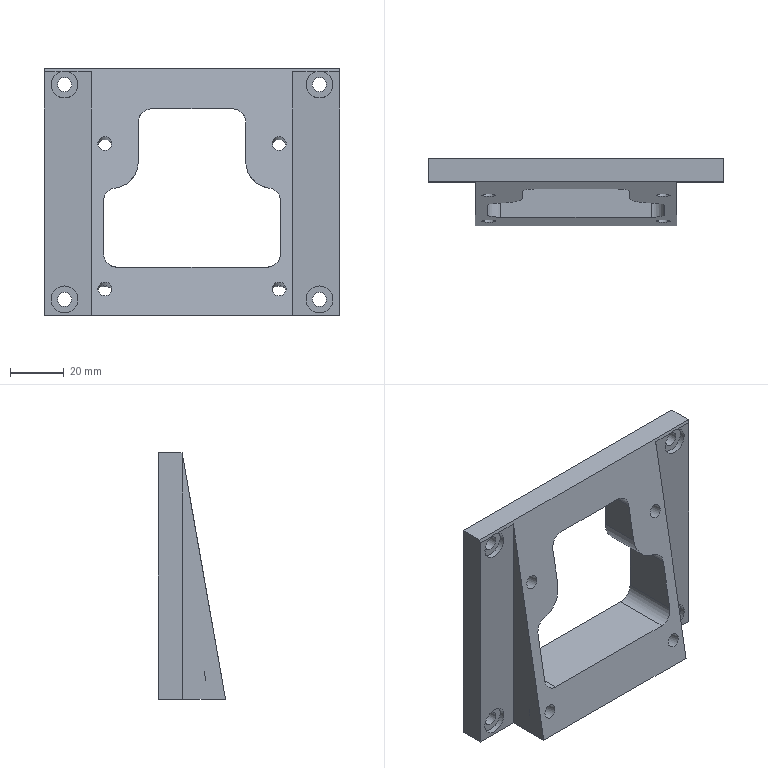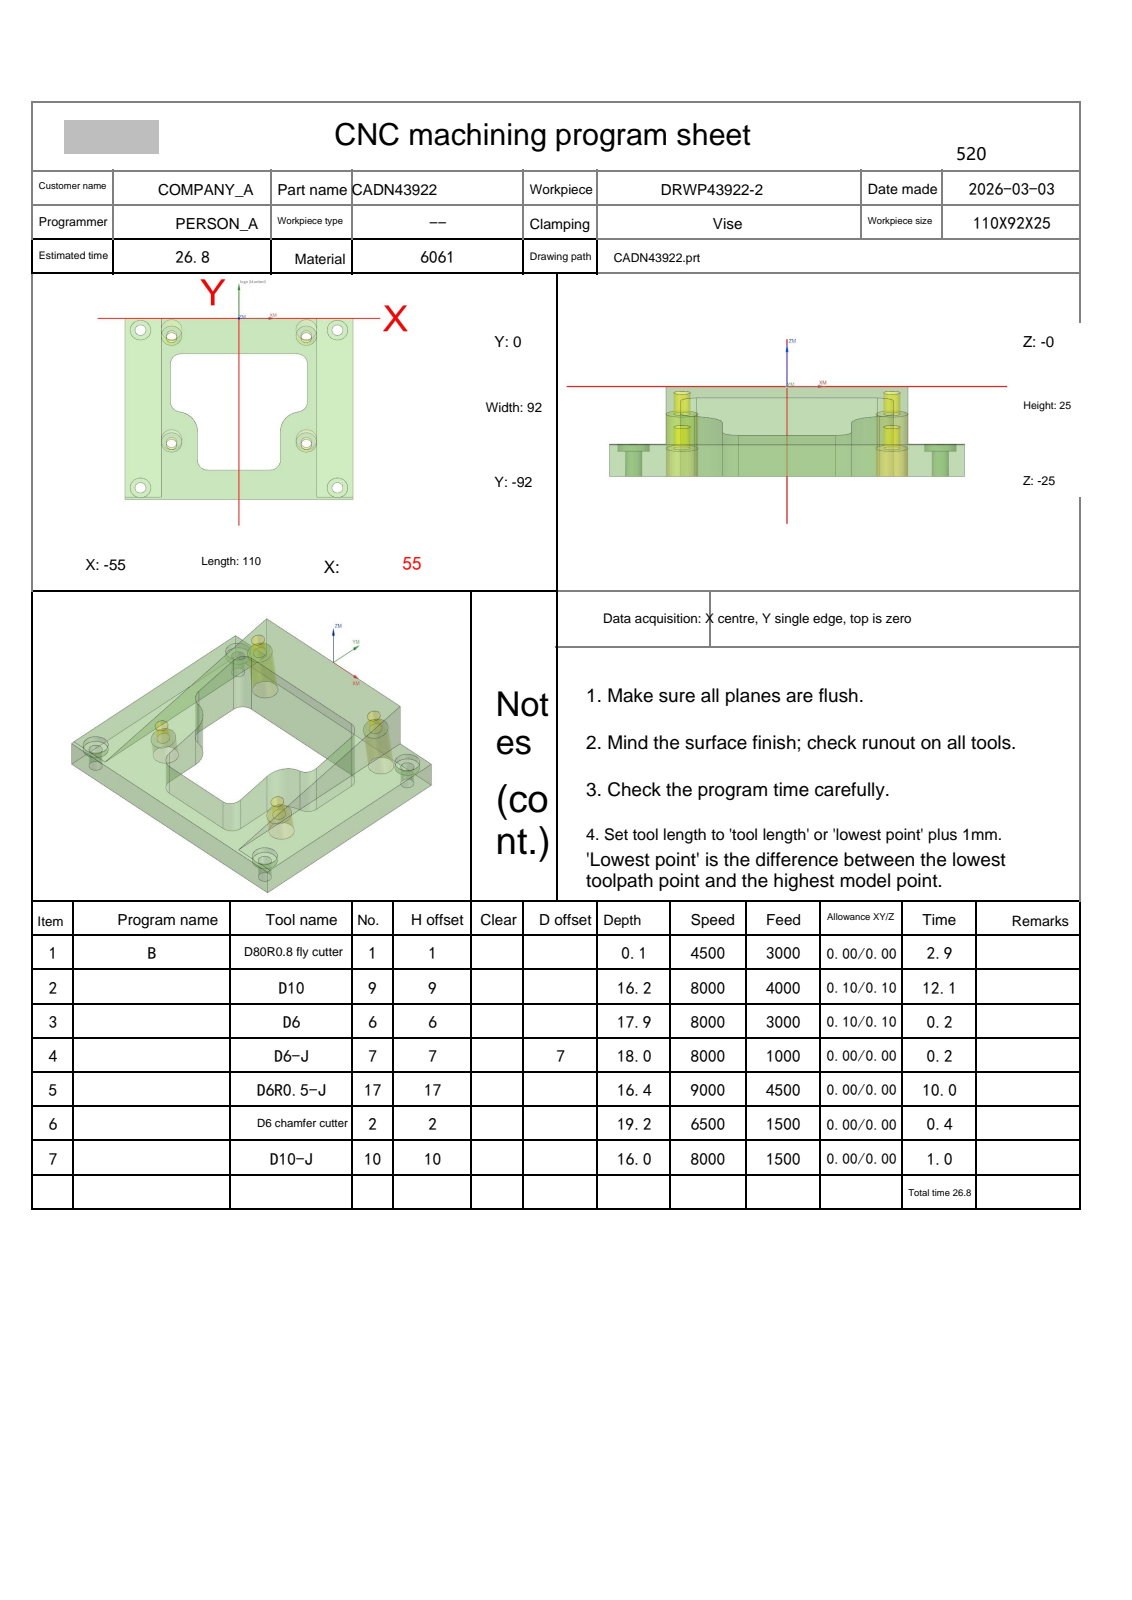NC program | NX | posted by the shop | part box 110 x 25 x 92 mm
Lines 183 to 1230 of 14355:
N2 T09 M06
(D10  D=10. R=0. H=09 ce=0.10 di=0.10)
G00 G90 G54 X7. Y-108. M03 S8000
G43 H09 Z14.5
M08
Z.509
G01 Z-.691 F4000.
Y-103.5
G03 X0.0 Y-96.5 I-7. J0.0
G01 X-51.
X-57.495
X-57.5
G02 X-58.003 Y-95.997 I0.0 J.503
G01 X-58. Y-95.943
X-58.001 Y3.993
Y3.998
G02 X-57.497 Y4.502 I.504 J0.0
G01 X-57.454 Y4.5
X-42.19
G02 X-37.512 Y6.5 I4.69 J-4.5
G01 X37.638 Y6.499
G02 X42.19 Y4.5 I-.138 J-6.499
G01 X57.495
X57.499
G02 X58.004 Y3.996 I0.0 J-.504
G01 X58.001 Y3.943
Y-95.994
Y-95.999
G02 X57.498 Y-96.502 I-.503 J0.0
G01 X57.454 Y-96.5
X-1.986
G02 X-2.799 Y-96.082 I.001 J1.
G01 X-7.201 Y-89.918
G03 X-8.014 Y-89.5 I-.813 J-.582
G01 X-50.003
G02 X-51. Y-88.502 I.002 J1.
G01 X-51.001 Y-11.861
G02 X-50.735 Y-11.182 I1. J0.0
G01 X-49.575 Y-9.925
G03 X-49.317 Y-9.373 I-.735 J.678
G02 X-46.837 Y-7.188 I2.48 J-.315
X-44.494 Y-8.817 I0.0 J-2.5
G01 X-42.645 Y-13.789
G02 X-42.488 Y-14.661 I-2.343 J-.871
X-44.988 Y-17.161 I-2.5 J0.0
X-47.331 Y-15.532 I0.0 J2.5
G01 X-48.77 Y-11.664
G03 X-49.071 Y-11.241 I-.937 J-.349
G01 X-50.637 Y-9.949
G02 X-51.001 Y-9.178 I.636 J.771
G01 Y-3.498
G02 X-50.003 Y-2.5 I1. J-.002
G01 X-44.998
G02 X-44. Y-3.497 I-.002 J-1.
G01 Y-3.904
X-44.002 Y-4.056
G03 X-37.5 Y-10.896 I6.849 J0.0
G01 X37.597 Y-10.893
G03 X44.001 Y-4.029 I-.476 J6.864
G01 Y-3.986
G03 X43.556 Y-3.287 I-.779 J-.005
G01 X43.2 Y-3.118
X43.02 Y-3.078
G03 X42.6 Y-3.498 I0.0 J-.42
G01 Y-3.921
X42.601 Y-4.029
G02 X37.5 Y-9.496 I-5.48 J0.0
G01 X-37.5
G02 X-42.602 Y-4.059 I.347 J5.438
G01 X-42.6 Y-3.921
Y-.444
G02 X-42.608 Y-.14 I5.438 J.304
X-42.592 Y.278 I5.446 J0.0
X-37.512 Y5.1 I5.093 J-.278
G01 X37.608 Y5.099
G02 X42.063 Y2.279 I-.108 J-5.099
X42.611 Y-.028 I-4.58 J-2.306
X42.6 Y-.356 I-5.128 J0.0
G01 Y-3.498
G03 X43.02 Y-3.918 I.42 J0.0
G01 X43.2 Y-3.877
X43.797 Y-3.594
G03 X44.018 Y-3.309 I-.172 J.361
G02 X44.998 Y-2.5 I.982 J-.191
G01 X50.003
G02 X51.001 Y-3.498 I-.002 J-1.
G01 Y-9.161
G02 X50.637 Y-9.932 I-1. J0.0
G01 X49.07 Y-11.225
G03 X48.769 Y-11.648 I.637 J-.771
G01 X47.329 Y-15.524
G02 X44.986 Y-17.153 I-2.343 J.871
X42.486 Y-14.653 I0.0 J2.5
X42.643 Y-13.782 I2.5 J0.0
G01 X44.493 Y-8.801
G02 X46.837 Y-7.172 I2.343 J-.871
X49.316 Y-9.356 I0.0 J-2.5
G03 X49.574 Y-9.908 I.992 J.126
G01 X50.735 Y-11.165
G02 X51.001 Y-11.844 I-.735 J-.678
G01 X51. Y-88.503
G02 X50.003 Y-89.5 I-1. J.002
G01 X-1.986
G02 X-2.799 Y-89.082 I.001 J1.
G01 X-7.201 Y-82.918
G03 X-8.014 Y-82.5 I-.813 J-.582
G01 X-43.003
G02 X-44. Y-81.503 I.003 J1.
G01 X-44.001 Y-17.703
G02 X-43.001 Y-16.705 I1. J-.003
X-42.609 Y-16.785 I0.0 J-1.
G03 X-37.678 Y-17.896 I5.459 J12.727
G01 X37.5
G03 X38.081 Y-17.876 I0.0 J8.4
X42.608 Y-16.779 I-.96 J13.847
G02 X43.001 Y-16.699 I.393 J-.92
X44.001 Y-17.696 I0.0 J-1.
G01 X44. Y-81.503
G02 X43.003 Y-82.5 I-1. J.003
G01 X-1.986
G02 X-2.799 Y-82.082 I.001 J1.
G01 X-7.201 Y-75.919
G03 X-8.014 Y-75.5 I-.813 J-.582
G01 X-36.003
G02 X-37. Y-74.503 I.003 J1.
G01 X-37.001 Y-25.893
G02 X-36.004 Y-24.896 I1. J-.003
G01 X36.004
G02 X37.001 Y-25.893 I-.003 J-1.
G01 X37. Y-74.503
G02 X36.003 Y-75.5 I-1. J.003
G01 X-1.986
G02 X-2.799 Y-75.082 I.001 J1.
G01 X-7.201 Y-68.919
G03 X-8.014 Y-68.5 I-.813 J-.582
G01 X-29.004
G02 X-30. Y-67.503 I.003 J1.
G01 X-30.001 Y-32.893
G02 X-29.004 Y-31.896 I1. J-.003
G01 X29.004
G02 X30.001 Y-32.893 I-.003 J-1.
G01 X30. Y-67.504
G02 X29.004 Y-68.5 I-1. J.003
G01 X-1.986
G02 X-2.799 Y-68.082 I0.0 J1.
G01 X-7.201 Y-61.919
G03 X-8.014 Y-61.5 I-.814 J-.582
G01 X-22.004
G02 X-23. Y-60.504 I.004 J1.
G01 X-23.001 Y-39.893
G02 X-22.004 Y-38.896 I1. J-.004
G01 X22.004
G02 X23.001 Y-39.893 I-.004 J-1.
G01 X23. Y-60.504
G02 X22.004 Y-61.5 I-1. J.004
G01 X-1.986
G02 X-2.799 Y-61.082 I0.0 J1.
G01 X-7.201 Y-54.919
G03 X-8.014 Y-54.5 I-.814 J-.582
G01 X-15.004
G02 X-16.001 Y-53.504 I.004 J1.
G01 Y-46.893
G02 X-15.004 Y-45.896 I1. J-.004
G01 X15.004
G02 X16.001 Y-46.893 I-.004 J-1.
G01 Y-53.504
G02 X15.004 Y-54.5 I-1. J.004
G01 X-5.
X-5.5
G03 X-12.5 Y-61.5 I0.0 J-7.
G01 Z.509
G00 Z3.
G01 X7. Y-108. F6000.
G00 Z-.183
G01 Z-1.383 F4000.
Y-103.5
G03 X0.0 Y-96.5 I-7. J0.0
G01 X-51.
X-57.495
X-57.5
G02 X-58.003 Y-95.997 I0.0 J.503
G01 X-58. Y-95.943
X-58.001 Y3.993
Y3.998
G02 X-57.497 Y4.502 I.504 J0.0
G01 X-57.454 Y4.5
X-42.19
G02 X-37.512 Y6.5 I4.69 J-4.5
G01 X37.628 Y6.499
G02 X42.19 Y4.5 I-.128 J-6.499
G01 X57.495
X57.499
G02 X58.004 Y3.996 I0.0 J-.504
G01 X58.001 Y3.943
Y-95.994
Y-95.999
G02 X57.498 Y-96.502 I-.503 J0.0
G01 X57.454 Y-96.5
X-5.
G02 X-5.971 Y-95.738 I0.0 J1.
G01 X-7.313 Y-90.262
G03 X-8.284 Y-89.5 I-.971 J-.239
G01 X-50.003
G02 X-51. Y-88.503 I.002 J1.
G01 X-51.001 Y-15.949
G02 X-50.736 Y-15.271 I1. J0.0
G01 X-49.576 Y-14.015
G03 X-49.319 Y-13.463 I-.735 J.678
G02 X-46.839 Y-11.276 I2.48 J-.313
X-44.496 Y-12.903 I0.0 J-2.5
G01 X-42.664 Y-17.819
G02 X-42.507 Y-18.692 I-2.343 J-.873
X-45.007 Y-21.192 I-2.5 J0.0
X-47.349 Y-19.565 I0.0 J2.5
G01 X-48.77 Y-15.753
G03 X-49.071 Y-15.33 I-.937 J-.349
G01 X-50.637 Y-14.039
G02 X-51.001 Y-13.268 I.636 J.772
G01 Y-3.497
G02 X-50.003 Y-2.5 I1. J-.002
G01 X-44.998
G02 X-44. Y-3.497 I-.002 J-1.
G01 Y-3.904
X-44.002 Y-4.059
X-44. Y-4.213
X-43.999 Y-7.906
X-43.973 Y-8.386
X-43.867 Y-9.275
G03 X-37.501 Y-14.817 I6.371 J.892
G01 X-34.608
G03 X-32.75 Y-14.55 I-.076 J7.123
G02 X-32.481 Y-14.513 I.269 J-.963
X-32.179 Y-14.56 I0.0 J-1.
G01 X-32.04 Y-14.604
G03 X-31.818 Y-14.656 I.427 J1.333
G01 X-30.927 Y-14.787
X-30.787 Y-14.8
X-30.392 Y-14.817
X30.456 Y-14.816
X30.787 Y-14.8
X30.93 Y-14.786
X31.82 Y-14.654
G03 X32.036 Y-14.604 I-.207 J1.385
G01 X32.177 Y-14.559
G02 X32.476 Y-14.513 I.299 J-.954
X32.746 Y-14.55 I0.0 J-1.
G03 X34.608 Y-14.817 I1.928 J6.82
G01 X37.5
G03 X44.004 Y-7.954 I-.37 J6.863
X44. Y-7.731 I-6.873 J0.0
G01 Y-4.151
X44.001 Y-3.985
G03 X43.556 Y-3.287 I-.779 J-.005
G01 X43.2 Y-3.118
X43.02 Y-3.077
G03 X42.6 Y-3.497 I0.0 J-.42
G01 Y-3.921
X42.601 Y-4.029
X42.6 Y-4.138
Y-7.755
G02 X42.604 Y-7.956 I-5.47 J-.201
X37.5 Y-13.417 I-5.473 J0.0
G01 X34.608
G02 X32.504 Y-12.987 I.065 J5.687
G01 X31.613 Y-13.269
X30.723 Y-13.402
X30.392 Y-13.417
X-30.392
X-30.723 Y-13.402
X-31.613 Y-13.271
X-32.504 Y-12.986
G02 X-34.608 Y-13.417 I-2.181 J5.291
G01 X-37.5
G02 X-42.477 Y-9.11 I.004 J5.033
G01 X-42.583 Y-8.221
X-42.6 Y-7.841
Y-4.197
X-42.602 Y-4.059
X-42.6 Y-3.921
Y-.444
G02 X-42.608 Y-.14 I5.438 J.304
X-42.592 Y.278 I5.446 J0.0
X-37.512 Y5.1 I5.092 J-.278
G01 X37.6 Y5.099
G02 X42.063 Y2.279 I-.1 J-5.099
X42.611 Y-.028 I-4.58 J-2.306
X42.6 Y-.356 I-5.128 J0.0
G01 Y-3.497
G03 X43.02 Y-3.917 I.42 J0.0
G01 X43.2 Y-3.877
X43.797 Y-3.594
G03 X44.018 Y-3.309 I-.172 J.361
G02 X44.997 Y-2.5 I.982 J-.191
G01 X50.003
G02 X51.001 Y-3.498 I-.002 J-1.
G01 Y-13.086
G02 X50.637 Y-13.857 I-1. J0.0
G01 X49.07 Y-15.15
G03 X48.77 Y-15.572 I.637 J-.771
G01 X47.33 Y-19.445
G02 X44.987 Y-21.074 I-2.343 J.871
X42.487 Y-18.574 I0.0 J2.5
X42.643 Y-17.703 I2.5 J0.0
G01 X44.494 Y-12.725
G02 X46.837 Y-11.096 I2.343 J-.871
X49.317 Y-13.281 I0.0 J-2.5
G03 X49.574 Y-13.833 I.992 J.126
G01 X50.735 Y-15.09
G02 X51.001 Y-15.769 I-.735 J-.678
G01 X51. Y-88.503
G02 X50.003 Y-89.5 I-1. J.002
G01 X-1.986
G02 X-2.799 Y-89.082 I.001 J1.
G01 X-7.201 Y-82.918
G03 X-8.014 Y-82.5 I-.813 J-.582
G01 X-43.003
G02 X-44. Y-81.503 I.003 J1.
G01 X-44.001 Y-21.723
G02 X-43.001 Y-20.726 I1. J-.003
X-42.622 Y-20.8 I0.0 J-1.
G03 X-37.504 Y-21.817 I5.126 J12.417
G01 X-34.571
G03 X-32.587 Y-21.661 I-.114 J14.123
G01 X-32.441 Y-21.65
X-32.298 Y-21.66
X-31.947 Y-21.712
G03 X-31.109 Y-21.793 I1.225 J8.31
G01 X31.109
G03 X31.963 Y-21.71 I-.386 J8.391
G01 X32.29 Y-21.661
X32.435 Y-21.65
X32.581 Y-21.661
G03 X34.576 Y-21.817 I2.093 J13.931
G01 X37.688
G03 X42.609 Y-20.7 I-.562 J13.862
G02 X43.001 Y-20.619 I.392 J-.92
X44.001 Y-21.617 I0.0 J-1.
G01 X44. Y-81.503
G02 X43.003 Y-82.5 I-1. J.003
G01 X-1.986
G02 X-2.799 Y-82.082 I.001 J1.
G01 X-7.201 Y-75.918
G03 X-8.014 Y-75.5 I-.813 J-.582
G01 X-36.004
G02 X-37. Y-74.503 I.003 J1.
G01 X-37.001 Y-29.814
G02 X-36.004 Y-28.817 I1. J-.003
G01 X-34.543
G03 X-32.577 Y-28.712 I-.142 J21.123
G01 X-32.48 Y-28.707
X-32.376 Y-28.713
G03 X-31.431 Y-28.785 I1.653 J15.311
G01 X-31.27 Y-28.793
X31.27
X31.431 Y-28.785
G03 X32.372 Y-28.713 I-.708 J15.384
G01 X32.476 Y-28.708
X32.573 Y-28.712
G03 X34.552 Y-28.817 I2.101 J20.982
G01 X36.004
G02 X37.001 Y-29.814 I-.003 J-1.
G01 X37. Y-74.503
G02 X36.004 Y-75.5 I-1. J.003
G01 X-1.986
G02 X-2.799 Y-75.082 I.001 J1.
G01 X-7.201 Y-68.919
G03 X-8.014 Y-68.5 I-.813 J-.582
G01 X-29.004
G02 X-30. Y-67.504 I.003 J1.
G01 X-30.001 Y-36.789
G02 X-29.004 Y-35.793 I1. J-.003
G01 X29.004
G02 X30.001 Y-36.789 I-.003 J-1.
G01 X30. Y-67.504
G02 X29.004 Y-68.5 I-1. J.003
G01 X-1.986
G02 X-2.799 Y-68.082 I0.0 J1.
G01 X-7.201 Y-61.919
G03 X-8.014 Y-61.5 I-.814 J-.582
G01 X-22.004
G02 X-23. Y-60.504 I.004 J1.
G01 X-23.001 Y-43.789
G02 X-22.004 Y-42.793 I1. J-.004
G01 X22.004
G02 X23.001 Y-43.789 I-.004 J-1.
G01 X23. Y-60.504
G02 X22.004 Y-61.5 I-1. J.004
G01 X-1.986
G02 X-2.799 Y-61.082 I0.0 J1.
G01 X-7.201 Y-54.919
G03 X-8.014 Y-54.5 I-.814 J-.582
G01 X-15.004
G02 X-16.001 Y-53.504 I.004 J1.
G01 Y-50.789
G02 X-15.004 Y-49.793 I1. J-.004
G01 X15.004
G02 X16.001 Y-50.789 I-.004 J-1.
G01 Y-53.504
G02 X15.004 Y-54.5 I-1. J.004
G01 X-5.
X-5.5
G03 X-12.5 Y-61.5 I0.0 J-7.
G01 Z-.183
G00 Z2.309
G01 X7. Y-108. F6000.
G00 Z-.874
G01 Z-2.074 F4000.
Y-103.5
G03 X0.0 Y-96.5 I-7. J0.0
G01 X-51.
X-57.495
X-57.5
G02 X-58.003 Y-95.997 I0.0 J.503
G01 X-58. Y-95.943
X-58.001 Y3.993
Y3.998
G02 X-57.497 Y4.502 I.504 J0.0
G01 X-57.454 Y4.5
X-42.19
G02 X-37.512 Y6.5 I4.69 J-4.5
G01 X37.617 Y6.499
G02 X42.19 Y4.5 I-.117 J-6.499
G01 X57.495
X57.499
G02 X58.004 Y3.996 I0.0 J-.504
G01 X58.001 Y3.943
Y-95.994
Y-95.999
G02 X57.498 Y-96.502 I-.503 J0.0
G01 X57.454 Y-96.5
X-5.
G02 X-5.971 Y-95.738 I0.0 J1.
G01 X-7.313 Y-90.262
G03 X-8.284 Y-89.5 I-.971 J-.239
G01 X-50.003
G02 X-51. Y-88.503 I.003 J1.
G01 X-51.001 Y-19.693
G02 X-50.735 Y-19.014 I1. J0.0
G01 X-49.574 Y-17.757
G03 X-49.317 Y-17.205 I-.735 J.678
G02 X-46.837 Y-15.02 I2.48 J-.315
X-44.494 Y-16.649 I0.0 J-2.5
G01 X-42.644 Y-21.626
G02 X-42.487 Y-22.497 I-2.343 J-.871
X-44.987 Y-24.997 I-2.5 J0.0
X-47.33 Y-23.368 I0.0 J2.5
G01 X-48.769 Y-19.496
G03 X-49.07 Y-19.073 I-.937 J-.348
G01 X-50.637 Y-17.781
G02 X-51.001 Y-17.01 I.636 J.771
G01 Y-3.497
G02 X-50.003 Y-2.5 I1. J-.003
G01 X-44.997
G02 X-44. Y-3.497 I-.003 J-1.
G01 Y-11.747
X-44.001 Y-11.884
G03 X-37.5 Y-18.738 I6.864 J0.0
G01 X37.5
G03 X44.001 Y-11.884 I-.362 J6.854
G01 X44. Y-11.747
Y-3.99
G03 X43.555 Y-3.286 I-.779 J0.0
G01 X43.2 Y-3.118
X43.02 Y-3.077
G03 X42.6 Y-3.497 I0.0 J-.42
G01 Y-11.762
X42.601 Y-11.886
G02 X37.5 Y-17.338 I-5.464 J0.0
G01 X-37.5
G02 X-42.601 Y-11.886 I.362 J5.452
G01 X-42.6 Y-11.762
Y-.444
G02 X-42.608 Y-.14 I5.438 J.304
X-42.592 Y.278 I5.446 J0.0
X-37.512 Y5.1 I5.092 J-.278
G01 X37.592 Y5.099
G02 X42.063 Y2.279 I-.092 J-5.099
X42.611 Y-.028 I-4.58 J-2.306
X42.6 Y-.356 I-5.128 J0.0
G01 Y-3.497
G03 X43.02 Y-3.917 I.42 J0.0
G01 X43.2 Y-3.877
X43.797 Y-3.593
G03 X44.018 Y-3.309 I-.172 J.361
G02 X44.997 Y-2.5 I.982 J-.191
G01 X50.003
G02 X51.001 Y-3.497 I-.003 J-1.
G01 Y-17.01
G02 X50.637 Y-17.781 I-1. J0.0
G01 X49.07 Y-19.074
G03 X48.77 Y-19.496 I.637 J-.771
G01 X47.33 Y-23.368
G02 X44.987 Y-24.997 I-2.343 J.871
X42.487 Y-22.497 I0.0 J2.5
X42.644 Y-21.626 I2.5 J0.0
G01 X44.494 Y-16.649
G02 X46.837 Y-15.02 I2.343 J-.871
X49.317 Y-17.205 I0.0 J-2.5
G03 X49.574 Y-17.757 I.992 J.126
G01 X50.735 Y-19.014
G02 X51.001 Y-19.693 I-.735 J-.678
G01 X51. Y-88.503
G02 X50.003 Y-89.5 I-1. J.003
G01 X-1.986
G02 X-2.799 Y-89.082 I.001 J1.
G01 X-7.201 Y-82.918
G03 X-8.014 Y-82.5 I-.813 J-.582
G01 X-43.003
G02 X-44. Y-81.503 I.003 J1.
G01 X-44.001 Y-25.539
G02 X-43.001 Y-24.542 I1. J-.003
X-42.609 Y-24.622 I0.0 J-1.
G03 X-37.685 Y-25.738 I5.474 J12.737
G01 X37.685
G03 X42.609 Y-24.622 I-.55 J13.853
G02 X43.001 Y-24.542 I.392 J-.92
X44.001 Y-25.539 I0.0 J-1.
G01 X44. Y-81.503
G02 X43.003 Y-82.5 I-1. J.003
G01 X-1.986
G02 X-2.799 Y-82.082 I.001 J1.
G01 X-7.201 Y-75.918
G03 X-8.014 Y-75.5 I-.813 J-.582
G01 X-36.004
G02 X-37. Y-74.503 I.003 J1.
G01 X-37.001 Y-33.734
G02 X-36.004 Y-32.738 I1. J-.003
G01 X36.004
G02 X37.001 Y-33.734 I-.003 J-1.
G01 X37. Y-74.504
G02 X36.004 Y-75.5 I-1. J.003
G01 X-1.986
G02 X-2.799 Y-75.082 I.001 J1.
G01 X-7.201 Y-68.918
G03 X-8.014 Y-68.5 I-.813 J-.582
G01 X-29.004
G02 X-30. Y-67.504 I.004 J1.
G01 X-30.001 Y-40.734
G02 X-29.004 Y-39.738 I1. J-.004
G01 X29.004
G02 X30.001 Y-40.734 I-.004 J-1.
G01 X30. Y-67.504
G02 X29.004 Y-68.5 I-1. J.004
G01 X-1.986
G02 X-2.799 Y-68.082 I0.0 J1.
G01 X-7.201 Y-61.919
G03 X-8.014 Y-61.5 I-.814 J-.582
G01 X-22.004
G02 X-23. Y-60.504 I.004 J1.
G01 X-23.001 Y-47.734
G02 X-22.004 Y-46.738 I1. J-.004
G01 X22.004
G02 X23.001 Y-47.734 I-.004 J-1.
G01 X23. Y-60.504
G02 X22.004 Y-61.5 I-1. J.004
G01 X-1.986
G02 X-2.799 Y-61.082 I0.0 J1.
G01 X-7.201 Y-54.919
G03 X-8.014 Y-54.5 I-.814 J-.581
G01 X-15.703
G02 X-16.001 Y-54.202 I.002 J.3
G01 Y-54.035
G02 X-15.703 Y-53.738 I.3 J-.002
G01 X15.703
G02 X16.001 Y-54.035 I-.002 J-.3
G01 Y-54.202
G02 X15.703 Y-54.5 I-.3 J.002
G01 X-5.
X-5.5
G03 X-12.5 Y-61.5 I0.0 J-7.
G01 Z-.874
G00 Z1.617
G01 X7. Y-108. F6000.
G00 Z-1.565
G01 Z-2.765 F4000.
Y-103.5
G03 X0.0 Y-96.5 I-7. J0.0
G01 X-51.
X-57.495
X-57.5
G02 X-58.003 Y-95.997 I0.0 J.503
G01 X-58. Y-95.943
X-58.001 Y3.993
Y3.998
G02 X-57.497 Y4.502 I.504 J0.0
G01 X-57.454 Y4.5
X-42.19
G02 X-37.512 Y6.5 I4.69 J-4.5
G01 X37.606 Y6.499
G02 X42.19 Y4.5 I-.106 J-6.499
G01 X57.495
X57.499
G02 X58.004 Y3.996 I0.0 J-.504
G01 X58.001 Y3.943
Y-95.994
Y-95.999
G02 X57.498 Y-96.502 I-.503 J0.0
G01 X57.454 Y-96.5
X-5.
G02 X-5.971 Y-95.738 I0.0 J1.
G01 X-7.313 Y-90.262
G03 X-8.284 Y-89.5 I-.971 J-.239
G01 X-50.003
G02 X-51. Y-88.503 I.003 J1.
G01 X-51.001 Y-23.796
G02 X-50.735 Y-23.117 I1. J0.0
G01 X-49.576 Y-21.861
G03 X-49.319 Y-21.309 I-.735 J.678
G02 X-46.839 Y-19.122 I2.48 J-.313
X-44.496 Y-20.749 I0.0 J-2.5
G01 X-42.665 Y-25.663
G02 X-42.507 Y-26.536 I-2.343 J-.873
X-45.007 Y-29.036 I-2.5 J0.0
X-47.35 Y-27.41 I0.0 J2.5
G01 X-48.77 Y-23.599
G03 X-49.071 Y-23.177 I-.937 J-.349
G01 X-50.637 Y-21.885
G02 X-51.001 Y-21.114 I.636 J.772
G01 Y-3.497
G02 X-50.004 Y-2.5 I1. J-.003
G01 X-44.997
G02 X-44. Y-3.497 I-.003 J-1.
G01 Y-11.747
X-44.001 Y-11.886
X-44. Y-12.025
X-43.998 Y-15.661
X-43.952 Y-16.383
X-43.882 Y-16.982
G03 X-37.506 Y-22.658 I6.376 J.743
G01 X37.519
G03 X43.941 Y-16.608 I0.0 J6.433
G01 X44. Y-15.577
Y-3.99
G03 X43.555 Y-3.286 I-.779 J0.0
G01 X43.2 Y-3.118
X43.02 Y-3.077
G03 X42.6 Y-3.497 I0.0 J-.42
G01 Y-15.577
X42.544 Y-16.524
G02 X37.519 Y-21.258 I-5.024 J.3
G01 X-37.506
G02 X-42.492 Y-16.82 I0.0 J5.019
G01 X-42.562 Y-16.221
X-42.6 Y-15.577
Y-12.01
X-42.601 Y-11.886
X-42.6 Y-11.762
Y-.444
G02 X-42.608 Y-.14 I5.438 J.304
X-42.592 Y.278 I5.446 J0.0
X-37.512 Y5.1 I5.092 J-.278
G01 X37.583 Y5.099
G02 X42.063 Y2.279 I-.083 J-5.099
X42.611 Y-.028 I-4.58 J-2.306
X42.6 Y-.356 I-5.128 J0.0
G01 Y-3.497
G03 X43.02 Y-3.917 I.42 J0.0
G01 X43.2 Y-3.877
X43.798 Y-3.593
G03 X44.018 Y-3.309 I-.172 J.361
G02 X44.997 Y-2.5 I.982 J-.191
G01 X50.004
G02 X51.001 Y-3.497 I-.003 J-1.
G01 Y-21.139
G02 X50.637 Y-21.911 I-1. J0.0
G01 X49.071 Y-23.201
G03 X48.771 Y-23.622 I.636 J-.772
G01 X47.35 Y-27.42
G02 X45.009 Y-29.044 I-2.342 J.876
X42.509 Y-26.544 I0.0 J2.5
X42.667 Y-25.668 I2.5 J0.0
G01 X44.5 Y-20.768
G02 X46.841 Y-19.144 I2.342 J-.876
X49.322 Y-21.334 I0.0 J-2.5
G03 X49.579 Y-21.888 I.992 J.124
G01 X50.736 Y-23.141
G02 X51.001 Y-23.82 I-.735 J-.678
G01 X51. Y-88.503
G02 X50.003 Y-89.5 I-1. J.003
G01 X-1.986
G02 X-2.799 Y-89.082 I.001 J1.
G01 X-7.201 Y-82.918
G03 X-8.014 Y-82.5 I-.813 J-.582
G01 X-43.004
G02 X-44. Y-81.503 I.003 J1.
G01 X-44.001 Y-29.567
G02 X-43.001 Y-28.57 I1. J-.003
X-42.622 Y-28.645 I0.0 J-1.
G03 X-37.506 Y-29.658 I5.116 J12.406
G01 X37.519
G03 X42.624 Y-28.651 I0.0 J13.433
G02 X43.001 Y-28.577 I.377 J-.926
X44.001 Y-29.574 I0.0 J-1.
G01 X44. Y-81.503
G02 X43.004 Y-82.5 I-1. J.003
G01 X-1.986
G02 X-2.799 Y-82.082 I.001 J1.
G01 X-7.201 Y-75.919
G03 X-8.014 Y-75.5 I-.813 J-.582
G01 X-36.004
G02 X-37. Y-74.504 I.003 J1.
G01 X-37.001 Y-37.655
G02 X-36.004 Y-36.658 I1. J-.003
G01 X36.004
G02 X37.001 Y-37.655 I-.003 J-1.
G01 X37. Y-74.504
G02 X36.004 Y-75.5 I-1. J.003
G01 X-1.986
G02 X-2.799 Y-75.082 I.001 J1.
G01 X-7.201 Y-68.918
G03 X-8.014 Y-68.5 I-.813 J-.582
G01 X-29.004
G02 X-30. Y-67.504 I.004 J1.
G01 X-30.001 Y-44.655
G02 X-29.004 Y-43.658 I1. J-.004
G01 X29.004
G02 X30.001 Y-44.655 I-.004 J-1.
G01 X30. Y-67.504
G02 X29.004 Y-68.5 I-1. J.004
G01 X-1.986
G02 X-2.799 Y-68.082 I0.0 J1.
G01 X-7.201 Y-61.919
G03 X-8.014 Y-61.5 I-.814 J-.582
G01 X-22.004
G02 X-23. Y-60.504 I.004 J1.
G01 X-23.001 Y-51.654
G02 X-22.004 Y-50.658 I1. J-.004
G01 X22.004
G02 X23.001 Y-51.654 I-.004 J-1.
G01 X23. Y-60.504
G02 X22.004 Y-61.5 I-1. J.004
G01 X-2.336
G02 X-3.043 Y-61.208 I0.0 J1.
G01 X-6.957 Y-57.293
G03 X-7.664 Y-57. I-.707 J-.707
G01 X-17.604
G02 X-18.502 Y-56.099 I.004 J.901
G01 X-18.501 Y-56.054
G02 X-17.604 Y-55.158 I.9 J-.004
G01 X17.604
G02 X18.502 Y-56.059 I-.004 J-.901
G01 X18.5 Y-56.104
G02 X17.604 Y-57. I-.9 J.004
G01 X-5.
X-5.5
G03 X-12.5 Y-64. I0.0 J-7.
G01 Z-1.565
G00 Z.926
G01 X7. Y-108. F6000.
G00 Z-2.257
G01 Z-3.457 F4000.
Y-103.5
G03 X0.0 Y-96.5 I-7. J0.0
G01 X-51.
X-57.495
X-57.5
G02 X-58.003 Y-95.997 I0.0 J.503
G01 X-58. Y-95.943
X-58.001 Y3.993
Y3.998
G02 X-57.497 Y4.502 I.504 J0.0
G01 X-57.454 Y4.5
X-42.19
G02 X-37.512 Y6.5 I4.69 J-4.5
G01 X37.606 Y6.499
G02 X42.19 Y4.5 I-.106 J-6.499
G01 X57.495
X57.499
G02 X58.004 Y3.996 I0.0 J-.504
G01 X58.001 Y3.943
Y-95.994
Y-95.999
G02 X57.498 Y-96.502 I-.503 J0.0
G01 X57.454 Y-96.5
X-5.
G02 X-5.971 Y-95.738 I0.0 J1.
G01 X-7.313 Y-90.262
G03 X-8.284 Y-89.5 I-.971 J-.239
G01 X-50.003
G02 X-51. Y-88.503 I.003 J1.
G01 X-51.001 Y-27.559
G02 X-50.735 Y-26.88 I1. J0.0
G01 X-49.575 Y-25.624
G03 X-49.318 Y-25.071 I-.735 J.678
G02 X-46.838 Y-22.886 I2.48 J-.314
X-44.495 Y-24.513 I0.0 J-2.5
G01 X-42.646 Y-29.479
G02 X-42.489 Y-30.352 I-2.343 J-.872
X-44.989 Y-32.852 I-2.5 J0.0
X-47.332 Y-31.224 I0.0 J2.5
G01 X-48.77 Y-27.362
G03 X-49.071 Y-26.939 I-.937 J-.349
G01 X-50.637 Y-25.648
G02 X-51.001 Y-24.876 I.636 J.771
G01 Y-3.497
G02 X-50.004 Y-2.5 I1. J-.003
G01 X-44.997
G02 X-44. Y-3.497 I-.003 J-1.
G01 Y-11.747
X-44.001 Y-11.886
X-44. Y-12.025
Y-19.583
X-44.002 Y-19.762
G03 X-37.5 Y-26.579 I6.824 J0.0
G01 X-32.012 Y-26.576
G03 X-27.616 Y-24.746 I-.503 J7.408
G02 X-26.961 Y-24.5 I.657 J-.754
G01 X26.926
G02 X27.602 Y-24.766 I-.003 J-1.
G03 X32.107 Y-26.579 I4.612 J4.956
G01 X37.5
G03 X44.002 Y-19.762 I-.322 J6.816
G01 X44. Y-19.583
Y-3.989
G03 X43.555 Y-3.286 I-.779 J0.0
G01 X43.2 Y-3.117
X43.02 Y-3.077
G03 X42.6 Y-3.497 I0.0 J-.42
G01 Y-19.603
X42.602 Y-19.764
G02 X37.5 Y-25.179 I-5.424 J0.0
G01 X32.107
G02 X28.497 Y-23.685 I.107 J5.368
G01 X28.189 Y-23.332
X27.925 Y-23.1
X-27.951
G02 X-32.107 Y-25.179 I-4.565 J3.932
G01 X-37.5
G02 X-42.602 Y-19.764 I.322 J5.414
G01 X-42.6 Y-19.603
Y-12.01
X-42.601 Y-11.886
X-42.6 Y-11.762
Y-.444
G02 X-42.608 Y-.14 I5.438 J.304
X-42.592 Y.278 I5.446 J0.0
X-37.512 Y5.1 I5.092 J-.278
G01 X37.583 Y5.099
G02 X42.063 Y2.279 I-.083 J-5.099
X42.611 Y-.028 I-4.58 J-2.306
X42.6 Y-.356 I-5.128 J0.0
G01 Y-3.497
G03 X43.02 Y-3.917 I.42 J0.0
G01 X43.2 Y-3.876
X43.798 Y-3.593
G03 X44.019 Y-3.308 I-.172 J.361
G02 X44.997 Y-2.5 I.981 J-.192
G01 X50.004
G02 X51.001 Y-3.497 I-.003 J-1.
G01 Y-24.876
G02 X50.637 Y-25.648 I-1. J0.0
G01 X49.07 Y-26.94
G03 X48.77 Y-27.362 I.636 J-.771
G01 X47.332 Y-31.224
G02 X44.989 Y-32.852 I-2.343 J.872
X42.489 Y-30.352 I0.0 J2.5
X42.646 Y-29.479 I2.5 J0.0
G01 X44.495 Y-24.513
G02 X46.838 Y-22.886 I2.343 J-.872
X49.318 Y-25.071 I0.0 J-2.5
G03 X49.575 Y-25.624 I.992 J.126
G01 X50.735 Y-26.88
G02 X51.001 Y-27.559 I-.735 J-.678
G01 X51. Y-88.503
G02 X50.003 Y-89.5 I-1. J.003
G01 X-1.986
G02 X-2.799 Y-89.082 I.001 J1.
G01 X-7.201 Y-82.918
G03 X-8.014 Y-82.5 I-.813 J-.582
G01 X-43.004
G02 X-44. Y-81.503 I.003 J1.
G01 X-44.001 Y-33.392
G02 X-43.001 Y-32.395 I1. J-.003
X-42.611 Y-32.474 I0.0 J-1.
G03 X-37.665 Y-33.579 I5.435 J12.711
G01 X-32.107
G03 X-31.538 Y-33.559 I0.0 J8.4
X-25.258 Y-31.634 I-.978 J14.392
G02 X-24.761 Y-31.5 I.5 J-.866
G01 X24.66
G02 X25.165 Y-31.639 I-.003 J-1.
G03 X32.052 Y-33.579 I7.048 J11.829
G01 X37.665
G03 X42.611 Y-32.474 I-.489 J13.815
G02 X43.001 Y-32.395 I.39 J-.921
X44.001 Y-33.392 I0.0 J-1.
G01 X44. Y-81.504
G02 X43.004 Y-82.5 I-1. J.003
G01 X-1.986
G02 X-2.799 Y-82.082 I.001 J1.
G01 X-7.201 Y-75.918
G03 X-8.014 Y-75.5 I-.813 J-.582
G01 X-36.004
G02 X-37. Y-74.504 I.004 J1.
G01 X-37.001 Y-41.575
G02 X-36.004 Y-40.579 I1. J-.004
G01 X-32.107
G03 X-31.063 Y-40.543 I0.0 J15.4
X-23.475 Y-38.592 I-1.452 J21.375
G02 X-23.06 Y-38.5 I.419 J-.908
G01 X22.932
G02 X23.351 Y-38.594 I-.004 J-1.
G03 X32.011 Y-40.579 I8.862 J18.784
G01 X36.004
G02 X37.001 Y-41.575 I-.004 J-1.
G01 X37. Y-74.504
G02 X36.004 Y-75.5 I-1. J.004
G01 X-1.986
G02 X-2.799 Y-75.082 I.001 J1.
G01 X-7.201 Y-68.919
G03 X-8.014 Y-68.5 I-.813 J-.582
G01 X-29.004
G02 X-30. Y-67.504 I.004 J1.
G01 X-30.001 Y-48.378
G02 X-29.124 Y-47.39 I1. J-.004
G03 X-21.984 Y-45.57 I-3.392 J28.222
G02 X-21.621 Y-45.5 I.367 J-.93
G01 X21.478
G02 X21.844 Y-45.571 I-.004 J-1.
G03 X29.116 Y-47.406 I10.37 J25.761
G02 X30.001 Y-48.396 I-.115 J-.993
G01 X30. Y-67.504
G02 X29.004 Y-68.5 I-1. J.004
G01 X-1.986
G02 X-2.799 Y-68.082 I0.0 J1.
G01 X-7.201 Y-61.919
G03 X-8.014 Y-61.5 I-.814 J-.582
G01 X-22.005
G02 X-23. Y-60.504 I.004 J1.
G01 X-23.001 Y-54.038
G02 X-22.293 Y-53.086 I1. J-.004
G03 X-20.677 Y-52.556 I-10.222 J33.918
G02 X-20.351 Y-52.5 I.33 J-.944
G01 X20.199
G02 X20.527 Y-52.557 I-.004 J-1.
G03 X22.29 Y-53.133 I11.687 J32.747
G02 X23.001 Y-54.087 I-.289 J-.957
G01 X23. Y-60.504
G02 X22.005 Y-61.5 I-1. J.004
G01 X-5.
X-5.5
G03 X-12.5 Y-68.5 I0.0 J-7.
G01 Z-2.257
G00 Z.235
G01 X7. Y-108. F6000.
G00 Z-2.948
G01 Z-4.148 F4000.
Y-103.5
G03 X0.0 Y-96.5 I-7. J0.0
G01 X-51.
X-57.495
X-57.5
G02 X-58.003 Y-95.997 I0.0 J.503
G01 X-58. Y-95.943
X-58.001 Y3.993
Y3.998
G02 X-57.497 Y4.502 I.504 J0.0
G01 X-57.454 Y4.5
X-42.19
G02 X-37.512 Y6.5 I4.69 J-4.5
G01 X37.577
G02 X42.19 Y4.5 I-.077 J-6.5
G01 X57.495
X57.499
G02 X58.004 Y3.996 I0.0 J-.504
G01 X58.001 Y3.943
Y-95.994
Y-95.999
G02 X57.498 Y-96.502 I-.503 J0.0
G01 X57.454 Y-96.5
X-5.
G02 X-5.971 Y-95.738 I0.0 J1.
G01 X-7.313 Y-90.262
G03 X-8.284 Y-89.5 I-.971 J-.239
G01 X-50.004
G02 X-51. Y-88.503 I.003 J1.
G01 X-51.001 Y-31.448
G02 X-50.735 Y-30.77 I1. J0.0
G01 X-49.574 Y-29.512
G03 X-49.316 Y-28.96 I-.735 J.678
G02 X-46.837 Y-26.776 I2.48 J-.316
X-44.493 Y-28.405 I0.0 J-2.5
G01 X-42.643 Y-33.386
G02 X-42.486 Y-34.256 I-2.343 J-.871
X-44.986 Y-36.756 I-2.5 J0.0
X-47.329 Y-35.127 I0.0 J2.5
G01 X-48.769 Y-31.252
G03 X-49.07 Y-30.829 I-.937 J-.348
G01 X-50.637 Y-29.536
G02 X-51.001 Y-28.765 I.636 J.771
G01 Y-3.497
G02 X-50.004 Y-2.5 I1. J-.003
G01 X-44.997
G02 X-44. Y-3.497 I-.003 J-1.
G01 Y-23.51
X-44.001 Y-23.634
G03 X-39.842 Y-29.952 I6.879 J0.0
X-37.5 Y-30.499 I2.712 J6.321
G01 X-33.
G03 X-26.664 Y-25.294 I-.06 J6.531
G02 X-25.689 Y-24.5 I.978 J-.206
G01 X25.721
G02 X26.689 Y-25.262 I-.003 J-1.
G03 X33. Y-30.499 I6.663 J1.608
G01 X37.596 Y-30.496
G03 X44.001 Y-23.634 I-.474 J6.862
G01 X44. Y-23.51
Y-3.989
G03 X43.555 Y-3.286 I-.779 J0.0
G01 X43.2 Y-3.117
X43.02 Y-3.077
G03 X42.6 Y-3.497 I0.0 J-.42
G01 Y-23.524
X42.601 Y-23.634
G02 X37.5 Y-29.099 I-5.479 J0.0
G01 X33.
G02 X27.898 Y-23.657 I.352 J5.443
G01 X27.9 Y-23.524
Y-23.1
X-27.9
Y-23.524
X-27.935 Y-24.221
G02 X-33. Y-29.099 I-5.125 J.253
G01 X-37.5
G02 X-42.601 Y-23.634 I.378 J5.466
G01 X-42.6 Y-23.524
Y-.444
G02 X-42.608 Y-.14 I5.438 J.304
X-42.592 Y.278 I5.446 J0.0
X-37.512 Y5.1 I5.092 J-.278
G01 X37.561
G02 X42.063 Y2.279 I-.061 J-5.1
X42.611 Y-.028 I-4.58 J-2.306
X42.6 Y-.356 I-5.128 J0.0
G01 Y-3.497
G03 X43.02 Y-3.917 I.42 J0.0
G01 X43.2 Y-3.876
X43.798 Y-3.593
G03 X44.019 Y-3.308 I-.172 J.361
G02 X44.997 Y-2.5 I.981 J-.192
G01 X50.004
G02 X51.001 Y-3.497 I-.003 J-1.
G01 Y-28.765
G02 X50.637 Y-29.536 I-1. J0.0
G01 X49.07 Y-30.829
G03 X48.769 Y-31.252 I.637 J-.771
G01 X47.329 Y-35.127
G02 X44.986 Y-36.756 I-2.343 J.871